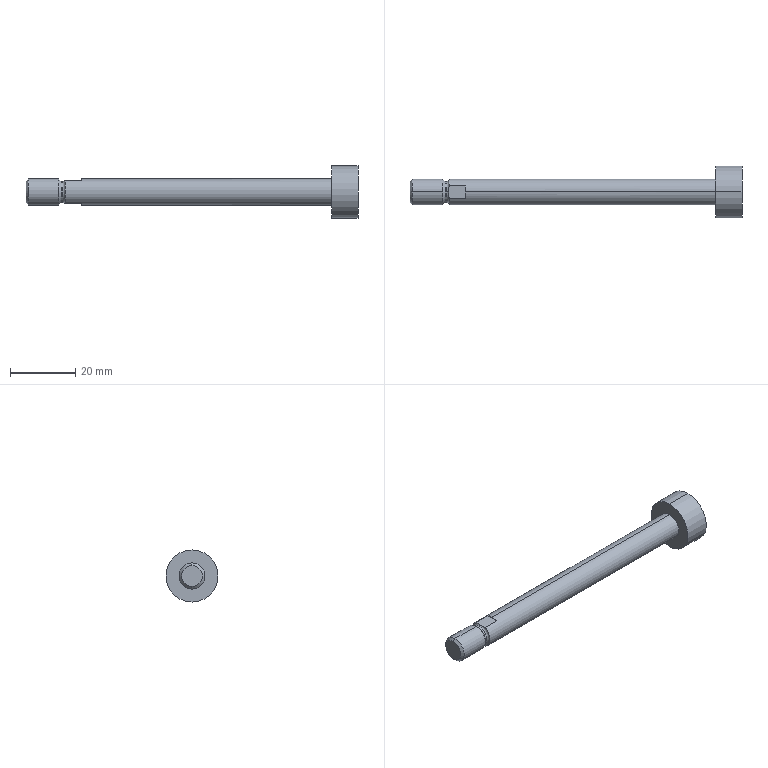Part | STEP file | 4935_DGS_16_1_P_k_HI | 1 solid | 23 faces | box 102 x 16 x 16 mm | volume 6287 mm3 | plane 9 | cylinder 8 | cone 4 | torus 2 | commonest cylinder face diameters 8 x4 6.466 x2 16 x2